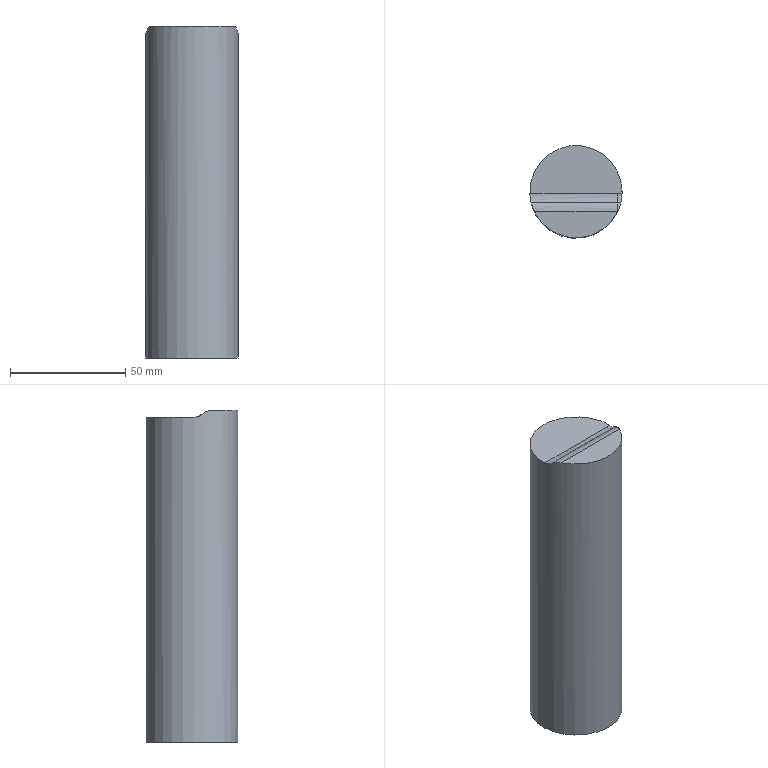Part | NX | features solid 2 | 1 solid | 8 faces | box 40 x 40 x 144.038 mm | volume 178325 mm3 | spline 6 | cylinder 1 | plane 1 | commonest cylinder face diameters 40 x1
STEP:
#1=CARTESIAN_POINT('',(579.982,-5.851,-10.126));
#2=VERTEX_POINT('',#1);
#3=CARTESIAN_POINT('',(577.981,-5.888,-10.126));
#4=VERTEX_POINT('',#3);
#5=CARTESIAN_POINT('',(577.981,-5.888,-10.126));
#6=CARTESIAN_POINT('',(578.648,-5.888,-10.126));
#7=CARTESIAN_POINT('',(579.315,-5.875,-10.126));
#8=CARTESIAN_POINT('',(579.982,-5.851,-10.126));
#9=B_SPLINE_CURVE_WITH_KNOTS('',3,(#5,#6,#7,#8),.UNSPECIFIED.,.F.,.F.,(4,4),(0.,0.05437),.UNSPECIFIED.);
#10=EDGE_CURVE('',#2,#4,#9,.F.);
#11=ORIENTED_EDGE('',*,*,#10,.T.);
#12=CARTESIAN_POINT('',(577.981,-9.844,-8.592));
#13=VERTEX_POINT('',#12);
#14=CARTESIAN_POINT('',(577.981,-9.844,-8.592));
#15=CARTESIAN_POINT('',(577.981,-8.768,-9.557));
#16=CARTESIAN_POINT('',(577.981,-7.333,-10.113));
#17=CARTESIAN_POINT('',(577.981,-5.888,-10.126));
#18=B_SPLINE_CURVE_WITH_KNOTS('',3,(#14,#15,#16,#17),.UNSPECIFIED.,.F.,.F.,(4,4),(0.,1.),.UNSPECIFIED.);
#19=EDGE_CURVE('',#4,#13,#18,.F.);
#20=ORIENTED_EDGE('',*,*,#19,.T.);
#21=CARTESIAN_POINT('',(579.409,-9.827,-8.591));
#22=VERTEX_POINT('',#21);
#23=CARTESIAN_POINT('',(579.409,-9.826,-8.592));
#24=CARTESIAN_POINT('',(578.933,-9.838,-8.592));
#25=CARTESIAN_POINT('',(578.457,-9.844,-8.592));
#26=CARTESIAN_POINT('',(577.981,-9.844,-8.592));
#27=B_SPLINE_CURVE_WITH_KNOTS('',3,(#23,#24,#25,#26),.UNSPECIFIED.,.F.,.F.,(4,4),(0.9639,1.),.UNSPECIFIED.);
#28=EDGE_CURVE('',#22,#13,#27,.T.);
#29=ORIENTED_EDGE('',*,*,#28,.F.);
#30=CARTESIAN_POINT('',(579.982,-5.851,-10.126));
#31=CARTESIAN_POINT('',(579.919,-7.324,-10.113));
#32=CARTESIAN_POINT('',(579.678,-8.744,-9.556));
#33=CARTESIAN_POINT('',(579.409,-9.826,-8.592));
#34=B_SPLINE_CURVE_WITH_KNOTS('',3,(#30,#31,#32,#33),.UNSPECIFIED.,.F.,.F.,(4,4),(0.,0.004403),.UNSPECIFIED.);
#35=EDGE_CURVE('',#2,#22,#34,.T.);
#36=ORIENTED_EDGE('',*,*,#35,.F.);
#37=EDGE_LOOP('',(#11,#20,#29,#36));
#38=FACE_BOUND('',#37,.T.);
#39=CARTESIAN_POINT('',(580.142,-9.803,-8.592));
#40=CARTESIAN_POINT('',(580.118,-9.158,-9.171));
#41=CARTESIAN_POINT('',(580.09,-8.408,-9.634));
#42=CARTESIAN_POINT('',(580.059,-7.582,-9.954));
#43=CARTESIAN_POINT('',(580.026,-6.717,-10.119));
#44=CARTESIAN_POINT('',(579.994,-5.85,-10.126));
#45=CARTESIAN_POINT('',(579.71,-9.819,-8.592));
#46=CARTESIAN_POINT('',(579.691,-9.174,-9.171));
#47=CARTESIAN_POINT('',(579.668,-8.424,-9.634));
#48=CARTESIAN_POINT('',(579.644,-7.598,-9.954));
#49=CARTESIAN_POINT('',(579.618,-6.732,-10.118));
#50=CARTESIAN_POINT('',(579.592,-5.865,-10.126));
#51=CARTESIAN_POINT('',(579.278,-9.831,-8.592));
#52=CARTESIAN_POINT('',(579.264,-9.186,-9.171));
#53=CARTESIAN_POINT('',(579.247,-8.436,-9.634));
#54=CARTESIAN_POINT('',(579.228,-7.609,-9.954));
#55=CARTESIAN_POINT('',(579.209,-6.744,-10.118));
#56=CARTESIAN_POINT('',(579.189,-5.877,-10.126));
#57=CARTESIAN_POINT('',(578.846,-9.839,-8.592));
#58=CARTESIAN_POINT('',(578.836,-9.194,-9.171));
#59=CARTESIAN_POINT('',(578.825,-8.444,-9.634));
#60=CARTESIAN_POINT('',(578.813,-7.617,-9.954));
#61=CARTESIAN_POINT('',(578.8,-6.751,-10.118));
#62=CARTESIAN_POINT('',(578.787,-5.884,-10.126));
#63=CARTESIAN_POINT('',(578.414,-9.844,-8.592));
#64=CARTESIAN_POINT('',(578.409,-9.198,-9.171));
#65=CARTESIAN_POINT('',(578.403,-8.448,-9.634));
#66=CARTESIAN_POINT('',(578.397,-7.621,-9.954));
#67=CARTESIAN_POINT('',(578.391,-6.755,-10.118));
#68=CARTESIAN_POINT('',(578.384,-5.888,-10.126));
#69=CARTESIAN_POINT('',(577.981,-9.844,-8.592));
#70=CARTESIAN_POINT('',(577.981,-9.198,-9.171));
#71=CARTESIAN_POINT('',(577.981,-8.448,-9.634));
#72=CARTESIAN_POINT('',(577.981,-7.621,-9.954));
#73=CARTESIAN_POINT('',(577.981,-6.755,-10.118));
#74=CARTESIAN_POINT('',(577.981,-5.888,-10.126));
#75=B_SPLINE_SURFACE_WITH_KNOTS('',5,5,((#39,#40,#41,#42,#43,#44),(#45,#46,#47,#48,#49,#50),(#51,#52,#53,#54,#55,#56),(#57,#58,#59,#60,#61,#62),(#63,#64,#65,#66,#67,#68),(#69,#70,#71,#72,#73,#74)),.UNSPECIFIED.,.F.,.F.,.F.,(6,6),(6,6),(0.9453,1.),(0.,1.),.PIECEWISE_BEZIER_KNOTS.);
#76=ADVANCED_FACE('',(#38),#75,.F.);
#77=CARTESIAN_POINT('',(540.02,-5.888,-10.126));
#78=VERTEX_POINT('',#77);
#79=CARTESIAN_POINT('',(577.981,-5.888,-10.126));
#80=CARTESIAN_POINT('',(565.328,-5.888,-10.126));
#81=CARTESIAN_POINT('',(552.674,-5.888,-10.126));
#82=CARTESIAN_POINT('',(540.02,-5.888,-10.126));
#83=B_SPLINE_CURVE_WITH_KNOTS('',3,(#79,#80,#81,#82),.UNSPECIFIED.,.F.,.F.,(4,4),(0.,0.09313),.UNSPECIFIED.);
#84=EDGE_CURVE('',#4,#78,#83,.T.);
#85=ORIENTED_EDGE('',*,*,#84,.F.);
#86=ORIENTED_EDGE('',*,*,#10,.F.);
#87=CARTESIAN_POINT('',(540.02,-5.888,-10.126));
#88=CARTESIAN_POINT('',(539.9,-3.202,-10.149));
#89=CARTESIAN_POINT('',(540.76,2.226,-10.195));
#90=CARTESIAN_POINT('',(545.151,9.207,-10.254));
#91=CARTESIAN_POINT('',(551.919,13.894,-10.294));
#92=CARTESIAN_POINT('',(559.98,15.549,-10.309));
#93=CARTESIAN_POINT('',(568.045,13.91,-10.295));
#94=CARTESIAN_POINT('',(574.828,9.23,-10.255));
#95=CARTESIAN_POINT('',(579.229,2.257,-10.195));
#96=CARTESIAN_POINT('',(580.096,-3.173,-10.149));
#97=CARTESIAN_POINT('',(579.982,-5.851,-10.126));
#98=B_SPLINE_CURVE_WITH_KNOTS('',3,(#87,#88,#89,#90,#91,#92,#93,#94,#95,#96,#97),.UNSPECIFIED.,.F.,.F.,(4,1,1,1,1,1,1,1,4),(0.005201,0.01323,0.02127,0.0293,0.03733,0.04536,0.05339,0.06143,0.06946),.UNSPECIFIED.);
#99=EDGE_CURVE('',#78,#2,#98,.T.);
#100=ORIENTED_EDGE('',*,*,#99,.F.);
#101=EDGE_LOOP('',(#85,#86,#100));
#102=FACE_BOUND('',#101,.T.);
#103=CARTESIAN_POINT('',(580.255,15.403,-10.307));
#104=CARTESIAN_POINT('',(539.754,15.403,-10.307));
#105=CARTESIAN_POINT('',(580.255,-5.888,-10.126));
#106=CARTESIAN_POINT('',(539.754,-5.888,-10.126));
#107=B_SPLINE_SURFACE_WITH_KNOTS('',1,1,((#103,#104),(#105,#106)),.PLANE_SURF.,.F.,.F.,.F.,(2,2),(2,2),(0.5799,0.9185),(0.06971,0.1047),.PIECEWISE_BEZIER_KNOTS.);
#108=ADVANCED_FACE('',(#102),#107,.F.);
#109=CARTESIAN_POINT('',(540.595,-9.844,-8.592));
#110=VERTEX_POINT('',#109);
#111=CARTESIAN_POINT('',(577.981,-9.844,-8.592));
#112=CARTESIAN_POINT('',(565.519,-9.844,-8.592));
#113=CARTESIAN_POINT('',(553.057,-9.844,-8.592));
#114=CARTESIAN_POINT('',(540.595,-9.844,-8.592));
#115=B_SPLINE_CURVE_WITH_KNOTS('',3,(#111,#112,#113,#114),.UNSPECIFIED.,.F.,.F.,(4,4),(0.,0.09172),.UNSPECIFIED.);
#116=EDGE_CURVE('',#13,#110,#115,.T.);
#117=ORIENTED_EDGE('',*,*,#116,.F.);
#118=ORIENTED_EDGE('',*,*,#19,.F.);
#119=ORIENTED_EDGE('',*,*,#84,.T.);
#120=CARTESIAN_POINT('',(540.595,-9.844,-8.592));
#121=CARTESIAN_POINT('',(540.327,-8.769,-9.556));
#122=CARTESIAN_POINT('',(540.085,-7.355,-10.113));
#123=CARTESIAN_POINT('',(540.02,-5.888,-10.126));
#124=B_SPLINE_CURVE_WITH_KNOTS('',3,(#120,#121,#122,#123),.UNSPECIFIED.,.F.,.F.,(4,4),(0.,0.004387),.UNSPECIFIED.);
#125=EDGE_CURVE('',#110,#78,#124,.T.);
#126=ORIENTED_EDGE('',*,*,#125,.F.);
#127=EDGE_LOOP('',(#117,#118,#119,#126));
#128=FACE_BOUND('',#127,.T.);
#129=CARTESIAN_POINT('',(577.981,-5.888,-10.126));
#130=CARTESIAN_POINT('',(539.792,-5.888,-10.126));
#131=CARTESIAN_POINT('',(577.981,-7.366,-10.113));
#132=CARTESIAN_POINT('',(539.792,-7.366,-10.113));
#133=CARTESIAN_POINT('',(577.981,-8.744,-9.579));
#134=CARTESIAN_POINT('',(539.792,-8.744,-9.579));
#135=CARTESIAN_POINT('',(577.981,-9.844,-8.592));
#136=CARTESIAN_POINT('',(539.792,-9.844,-8.592));
#137=(BOUNDED_SURFACE()B_SPLINE_SURFACE(3,1,((#129,#130),(#131,#132),(#133,#134),(#135,#136)),.CYLINDRICAL_SURF.,.F.,.F.,.F.)B_SPLINE_SURFACE_WITH_KNOTS((4,4),(2,2),(0.,1.),(0.,0.09369),.PIECEWISE_BEZIER_KNOTS.)GEOMETRIC_REPRESENTATION_ITEM()RATIONAL_B_SPLINE_SURFACE(((1.,1.),(0.9569,0.9569),(0.9569,0.9569),(1.,1.)))REPRESENTATION_ITEM('')SURFACE());
#138=ADVANCED_FACE('',(#128),#137,.F.);
#139=CARTESIAN_POINT('',(577.98,-13.777,-7.058));
#140=VERTEX_POINT('',#139);
#141=CARTESIAN_POINT('',(542.04,-13.799,-7.058));
#142=VERTEX_POINT('',#141);
#143=CARTESIAN_POINT('',(577.981,-13.799,-7.058));
#144=CARTESIAN_POINT('',(566.001,-13.799,-7.058));
#145=CARTESIAN_POINT('',(554.02,-13.799,-7.058));
#146=CARTESIAN_POINT('',(542.04,-13.799,-7.058));
#147=B_SPLINE_CURVE_WITH_KNOTS('',3,(#143,#144,#145,#146),.UNSPECIFIED.,.F.,.F.,(4,4),(0.,0.08817),.UNSPECIFIED.);
#148=EDGE_CURVE('',#140,#142,#147,.T.);
#149=ORIENTED_EDGE('',*,*,#148,.F.);
#150=CARTESIAN_POINT('',(577.981,-9.844,-8.592));
#151=CARTESIAN_POINT('',(577.981,-10.896,-7.647));
#152=CARTESIAN_POINT('',(577.981,-12.385,-7.07));
#153=CARTESIAN_POINT('',(577.981,-13.799,-7.058));
#154=B_SPLINE_CURVE_WITH_KNOTS('',3,(#150,#151,#152,#153),.UNSPECIFIED.,.F.,.F.,(4,4),(0.,1.),.UNSPECIFIED.);
#155=EDGE_CURVE('',#13,#140,#154,.T.);
#156=ORIENTED_EDGE('',*,*,#155,.F.);
#157=ORIENTED_EDGE('',*,*,#116,.T.);
#158=CARTESIAN_POINT('',(542.04,-13.799,-7.058));
#159=CARTESIAN_POINT('',(541.363,-12.419,-7.07));
#160=CARTESIAN_POINT('',(540.877,-10.97,-7.581));
#161=CARTESIAN_POINT('',(540.595,-9.844,-8.592));
#162=B_SPLINE_CURVE_WITH_KNOTS('',3,(#158,#159,#160,#161),.UNSPECIFIED.,.F.,.F.,(4,4),(0.,0.004545),.UNSPECIFIED.);
#163=EDGE_CURVE('',#142,#110,#162,.T.);
#164=ORIENTED_EDGE('',*,*,#163,.F.);
#165=EDGE_LOOP('',(#149,#156,#157,#164));
#166=FACE_BOUND('',#165,.T.);
#167=CARTESIAN_POINT('',(577.981,-9.844,-8.592));
#168=CARTESIAN_POINT('',(540.371,-9.844,-8.592));
#169=CARTESIAN_POINT('',(577.981,-10.944,-7.605));
#170=CARTESIAN_POINT('',(540.371,-10.944,-7.605));
#171=CARTESIAN_POINT('',(577.981,-12.321,-7.071));
#172=CARTESIAN_POINT('',(540.371,-12.321,-7.071));
#173=CARTESIAN_POINT('',(577.981,-13.799,-7.058));
#174=CARTESIAN_POINT('',(540.371,-13.799,-7.058));
#175=(BOUNDED_SURFACE()B_SPLINE_SURFACE(3,1,((#167,#168),(#169,#170),(#171,#172),(#173,#174)),.CYLINDRICAL_SURF.,.F.,.F.,.F.)B_SPLINE_SURFACE_WITH_KNOTS((4,4),(2,2),(0.,1.),(0.,0.09227),.PIECEWISE_BEZIER_KNOTS.)GEOMETRIC_REPRESENTATION_ITEM()RATIONAL_B_SPLINE_SURFACE(((1.,1.),(0.9569,0.9569),(0.9569,0.9569),(1.,1.)))REPRESENTATION_ITEM('')SURFACE());
#176=ADVANCED_FACE('',(#166),#175,.F.);
#177=ORIENTED_EDGE('',*,*,#148,.T.);
#178=CARTESIAN_POINT('',(577.964,-13.791,-7.058));
#179=CARTESIAN_POINT('',(576.336,-17.119,-7.03));
#180=CARTESIAN_POINT('',(571.139,-22.882,-6.98));
#181=CARTESIAN_POINT('',(560.01,-26.059,-6.953));
#182=CARTESIAN_POINT('',(548.865,-22.884,-6.98));
#183=CARTESIAN_POINT('',(543.672,-17.131,-7.03));
#184=CARTESIAN_POINT('',(542.04,-13.799,-7.058));
#185=B_SPLINE_CURVE_WITH_KNOTS('',3,(#178,#179,#180,#181,#182,#183,#184),.UNSPECIFIED.,.F.,.F.,(4,1,1,1,4),(0.0716,0.0827,0.0938,0.1049,0.116),.UNSPECIFIED.);
#186=EDGE_CURVE('',#140,#142,#185,.T.);
#187=ORIENTED_EDGE('',*,*,#186,.F.);
#188=EDGE_LOOP('',(#177,#187));
#189=FACE_BOUND('',#188,.T.);
#190=CARTESIAN_POINT('',(578.197,-13.723,-7.059));
#191=CARTESIAN_POINT('',(541.824,-13.723,-7.059));
#192=CARTESIAN_POINT('',(578.197,-25.103,-6.961));
#193=CARTESIAN_POINT('',(541.824,-25.103,-6.961));
#194=B_SPLINE_SURFACE_WITH_KNOTS('',1,1,((#190,#191),(#192,#193)),.PLANE_SURF.,.F.,.F.,.F.,(2,2),(2,2),(0.6217,0.7643),(0.06745,0.09447),.PIECEWISE_BEZIER_KNOTS.);
#195=ADVANCED_FACE('',(#189),#194,.F.);
#196=ORIENTED_EDGE('',*,*,#28,.T.);
#197=ORIENTED_EDGE('',*,*,#155,.T.);
#198=CARTESIAN_POINT('',(579.411,-9.82,-8.598));
#199=CARTESIAN_POINT('',(579.132,-10.942,-7.595));
#200=CARTESIAN_POINT('',(578.651,-12.381,-7.08));
#201=CARTESIAN_POINT('',(577.981,-13.756,-7.059));
#202=B_SPLINE_CURVE_WITH_KNOTS('',3,(#198,#199,#200,#201),.UNSPECIFIED.,.F.,.F.,(4,4),(0.,0.00457),.UNSPECIFIED.);
#203=EDGE_CURVE('',#22,#140,#202,.T.);
#204=ORIENTED_EDGE('',*,*,#203,.F.);
#205=EDGE_LOOP('',(#196,#197,#204));
#206=FACE_BOUND('',#205,.T.);
#207=CARTESIAN_POINT('',(579.518,-13.78,-7.058));
#208=CARTESIAN_POINT('',(579.497,-12.911,-7.066));
#209=CARTESIAN_POINT('',(579.475,-12.044,-7.23));
#210=CARTESIAN_POINT('',(579.454,-11.216,-7.552));
#211=CARTESIAN_POINT('',(579.435,-10.465,-8.016));
#212=CARTESIAN_POINT('',(579.419,-9.819,-8.598));
#213=CARTESIAN_POINT('',(579.211,-13.788,-7.058));
#214=CARTESIAN_POINT('',(579.194,-12.919,-7.065));
#215=CARTESIAN_POINT('',(579.176,-12.052,-7.23));
#216=CARTESIAN_POINT('',(579.16,-11.224,-7.552));
#217=CARTESIAN_POINT('',(579.145,-10.472,-8.016));
#218=CARTESIAN_POINT('',(579.132,-9.827,-8.597));
#219=CARTESIAN_POINT('',(578.904,-13.793,-7.058));
#220=CARTESIAN_POINT('',(578.891,-12.925,-7.065));
#221=CARTESIAN_POINT('',(578.878,-12.057,-7.23));
#222=CARTESIAN_POINT('',(578.865,-11.229,-7.552));
#223=CARTESIAN_POINT('',(578.854,-10.478,-8.016));
#224=CARTESIAN_POINT('',(578.844,-9.832,-8.597));
#225=CARTESIAN_POINT('',(578.596,-13.797,-7.058));
#226=CARTESIAN_POINT('',(578.588,-12.928,-7.065));
#227=CARTESIAN_POINT('',(578.579,-12.061,-7.23));
#228=CARTESIAN_POINT('',(578.571,-11.233,-7.552));
#229=CARTESIAN_POINT('',(578.563,-10.482,-8.016));
#230=CARTESIAN_POINT('',(578.557,-9.836,-8.597));
#231=CARTESIAN_POINT('',(578.289,-13.799,-7.058));
#232=CARTESIAN_POINT('',(578.284,-12.93,-7.065));
#233=CARTESIAN_POINT('',(578.28,-12.063,-7.23));
#234=CARTESIAN_POINT('',(578.276,-11.235,-7.552));
#235=CARTESIAN_POINT('',(578.272,-10.483,-8.016));
#236=CARTESIAN_POINT('',(578.269,-9.837,-8.597));
#237=CARTESIAN_POINT('',(577.981,-13.799,-7.058));
#238=CARTESIAN_POINT('',(577.981,-12.93,-7.065));
#239=CARTESIAN_POINT('',(577.981,-12.063,-7.23));
#240=CARTESIAN_POINT('',(577.981,-11.235,-7.552));
#241=CARTESIAN_POINT('',(577.981,-10.483,-8.016));
#242=CARTESIAN_POINT('',(577.981,-9.837,-8.597));
#243=B_SPLINE_SURFACE_WITH_KNOTS('',5,5,((#207,#208,#209,#210,#211,#212),(#213,#214,#215,#216,#217,#218),(#219,#220,#221,#222,#223,#224),(#225,#226,#227,#228,#229,#230),(#231,#232,#233,#234,#235,#236),(#237,#238,#239,#240,#241,#242)),.UNSPECIFIED.,.F.,.F.,.F.,(6,6),(6,6),(0.9636,1.),(0.,1.),.PIECEWISE_BEZIER_KNOTS.);
#244=ADVANCED_FACE('',(#206),#243,.F.);
#245=CARTESIAN_POINT('',(580.,-5.,-151.));
#246=VERTEX_POINT('',#245);
#247=CARTESIAN_POINT('',(560.,-5.,-151.));
#248=DIRECTION('',(0.,0.,1.));
#249=DIRECTION('',(1.,0.,0.));
#250=AXIS2_PLACEMENT_3D('',#247,#248,#249);
#251=CIRCLE('',#250,20.);
#252=EDGE_CURVE('',#246,#246,#251,.T.);
#253=ORIENTED_EDGE('',*,*,#252,.T.);
#254=EDGE_LOOP('',(#253));
#255=FACE_BOUND('',#254,.T.);
#256=ORIENTED_EDGE('',*,*,#203,.T.);
#257=ORIENTED_EDGE('',*,*,#186,.T.);
#258=ORIENTED_EDGE('',*,*,#163,.T.);
#259=ORIENTED_EDGE('',*,*,#125,.T.);
#260=ORIENTED_EDGE('',*,*,#99,.T.);
#261=ORIENTED_EDGE('',*,*,#35,.T.);
#262=EDGE_LOOP('',(#256,#257,#258,#259,#260,#261));
#263=FACE_BOUND('',#262,.T.);
#264=CARTESIAN_POINT('',(560.,-5.,40.));
#265=DIRECTION('',(0.,0.,-1.));
#266=DIRECTION('',(-1.,0.,0.));
#267=AXIS2_PLACEMENT_3D('',#264,#265,#266);
#268=CYLINDRICAL_SURFACE('',#267,20.);
#269=ADVANCED_FACE('',(#255,#263),#268,.T.);
#270=ORIENTED_EDGE('',*,*,#252,.F.);
#271=EDGE_LOOP('',(#270));
#272=FACE_BOUND('',#271,.T.);
#273=CARTESIAN_POINT('',(560.,-5.,-151.));
#274=DIRECTION('',(0.,0.,1.));
#275=DIRECTION('',(1.,0.,0.));
#276=AXIS2_PLACEMENT_3D('',#273,#274,#275);
#277=PLANE('',#276);
#278=ADVANCED_FACE('',(#272),#277,.F.);
#279=CLOSED_SHELL('',(#76,#108,#138,#176,#195,#244,#269,#278));
#280=MANIFOLD_SOLID_BREP('',#279);
#281=(LENGTH_UNIT()NAMED_UNIT(*)SI_UNIT(.MILLI.,.METRE.));
#282=UNCERTAINTY_MEASURE_WITH_UNIT(LENGTH_MEASURE(0.09481),#281,'','');
#283=(NAMED_UNIT(*)PLANE_ANGLE_UNIT()SI_UNIT($,.RADIAN.));
#284=(NAMED_UNIT(*)SI_UNIT($,.STERADIAN.)SOLID_ANGLE_UNIT());
#285=(GEOMETRIC_REPRESENTATION_CONTEXT(3)GLOBAL_UNCERTAINTY_ASSIGNED_CONTEXT((#282))GLOBAL_UNIT_ASSIGNED_CONTEXT((#281,#283,#284))REPRESENTATION_CONTEXT('',''));
#286=ADVANCED_BREP_SHAPE_REPRESENTATION('',(#280),#285);